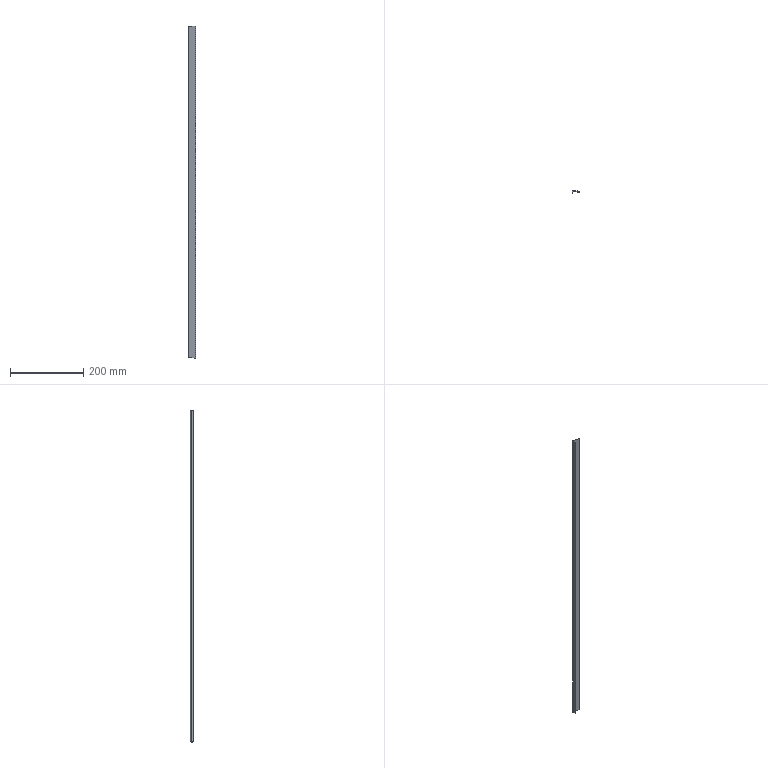Part | STEP file | 750078466 | 1 solid | 10 faces | box 19.319 x 9.272 x 903.6 mm | volume 29323 mm3 | plane 8 | cylinder 2 | commonest cylinder face diameters 2.4 x1 4.8 x1
STEP:
#1=CARTESIAN_POINT('',(19.008,3.665,451.8));
#2=VERTEX_POINT('',#1);
#3=CARTESIAN_POINT('',(19.008,3.665,-451.8));
#4=VERTEX_POINT('',#3);
#5=CARTESIAN_POINT('',(19.008,3.665,451.8));
#6=DIRECTION('',(0.,0.,-1.));
#7=VECTOR('',#6,1000.);
#8=LINE('',#5,#7);
#9=EDGE_CURVE('',#2,#4,#8,.T.);
#10=ORIENTED_EDGE('',*,*,#9,.F.);
#11=CARTESIAN_POINT('',(2.711,8.031,451.8));
#12=VERTEX_POINT('',#11);
#13=CARTESIAN_POINT('',(-0.3106,8.841,451.8));
#14=DIRECTION('',(0.9659,-0.2588,0.));
#15=VECTOR('',#14,1000.);
#16=LINE('',#13,#15);
#17=EDGE_CURVE('',#12,#2,#16,.T.);
#18=ORIENTED_EDGE('',*,*,#17,.F.);
#19=CARTESIAN_POINT('',(2.711,8.031,-451.8));
#20=VERTEX_POINT('',#19);
#21=CARTESIAN_POINT('',(2.711,8.031,451.8));
#22=DIRECTION('',(0.,0.,1.));
#23=VECTOR('',#22,1000.);
#24=LINE('',#21,#23);
#25=EDGE_CURVE('',#20,#12,#24,.T.);
#26=ORIENTED_EDGE('',*,*,#25,.F.);
#27=CARTESIAN_POINT('',(-0.3106,8.841,-451.8));
#28=DIRECTION('',(-0.9659,0.2588,0.));
#29=VECTOR('',#28,1000.);
#30=LINE('',#27,#29);
#31=EDGE_CURVE('',#4,#20,#30,.T.);
#32=ORIENTED_EDGE('',*,*,#31,.F.);
#33=EDGE_LOOP('',(#10,#18,#26,#32));
#34=FACE_OUTER_BOUND('',#33,.T.);
#35=CARTESIAN_POINT('',(-0.3106,8.841,451.8));
#36=DIRECTION('',(0.2588,0.9659,0.));
#37=DIRECTION('',(-0.9659,0.2588,0.));
#38=AXIS2_PLACEMENT_3D('',#35,#36,#37);
#39=PLANE('',#38);
#40=ADVANCED_FACE('',(#34),#39,.F.);
#41=CARTESIAN_POINT('',(3.021,9.19,-451.8));
#42=VERTEX_POINT('',#41);
#43=CARTESIAN_POINT('',(0.,6.872,-451.8));
#44=VERTEX_POINT('',#43);
#45=CARTESIAN_POINT('',(2.4,6.872,-451.8));
#46=DIRECTION('',(0.,0.,1.));
#47=DIRECTION('',(-1.,0.,0.));
#48=AXIS2_PLACEMENT_3D('',#45,#46,#47);
#49=CIRCLE('',#48,2.4);
#50=EDGE_CURVE('',#42,#44,#49,.T.);
#51=ORIENTED_EDGE('',*,*,#50,.F.);
#52=CARTESIAN_POINT('',(19.319,4.824,-451.8));
#53=VERTEX_POINT('',#52);
#54=CARTESIAN_POINT('',(19.319,4.824,-451.8));
#55=DIRECTION('',(-0.9659,0.2588,0.));
#56=VECTOR('',#55,1000.);
#57=LINE('',#54,#56);
#58=EDGE_CURVE('',#53,#42,#57,.T.);
#59=ORIENTED_EDGE('',*,*,#58,.F.);
#60=CARTESIAN_POINT('',(19.008,3.665,-451.8));
#61=DIRECTION('',(0.2588,0.9659,0.));
#62=VECTOR('',#61,1000.);
#63=LINE('',#60,#62);
#64=EDGE_CURVE('',#4,#53,#63,.T.);
#65=ORIENTED_EDGE('',*,*,#64,.F.);
#66=ORIENTED_EDGE('',*,*,#31,.T.);
#67=CARTESIAN_POINT('',(1.2,6.872,-451.8));
#68=VERTEX_POINT('',#67);
#69=CARTESIAN_POINT('',(2.4,6.872,-451.8));
#70=DIRECTION('',(0.,0.,-1.));
#71=DIRECTION('',(-1.,0.,0.));
#72=AXIS2_PLACEMENT_3D('',#69,#70,#71);
#73=CIRCLE('',#72,1.2);
#74=EDGE_CURVE('',#68,#20,#73,.T.);
#75=ORIENTED_EDGE('',*,*,#74,.F.);
#76=CARTESIAN_POINT('',(1.2,0.,-451.8));
#77=VERTEX_POINT('',#76);
#78=CARTESIAN_POINT('',(1.2,0.,-451.8));
#79=DIRECTION('',(0.,1.,0.));
#80=VECTOR('',#79,1000.);
#81=LINE('',#78,#80);
#82=EDGE_CURVE('',#77,#68,#81,.T.);
#83=ORIENTED_EDGE('',*,*,#82,.F.);
#84=CARTESIAN_POINT('',(0.,0.,-451.8));
#85=VERTEX_POINT('',#84);
#86=CARTESIAN_POINT('',(0.,0.,-451.8));
#87=DIRECTION('',(-1.,0.,0.));
#88=VECTOR('',#87,1000.);
#89=LINE('',#86,#88);
#90=EDGE_CURVE('',#77,#85,#89,.T.);
#91=ORIENTED_EDGE('',*,*,#90,.T.);
#92=CARTESIAN_POINT('',(0.,0.,-451.8));
#93=DIRECTION('',(0.,-1.,0.));
#94=VECTOR('',#93,1000.);
#95=LINE('',#92,#94);
#96=EDGE_CURVE('',#44,#85,#95,.T.);
#97=ORIENTED_EDGE('',*,*,#96,.F.);
#98=EDGE_LOOP('',(#51,#59,#65,#66,#75,#83,#91,#97));
#99=FACE_OUTER_BOUND('',#98,.T.);
#100=CARTESIAN_POINT('',(0.,0.,-451.8));
#101=DIRECTION('',(0.,0.,1.));
#102=DIRECTION('',(1.,0.,0.));
#103=AXIS2_PLACEMENT_3D('',#100,#101,#102);
#104=PLANE('',#103);
#105=ADVANCED_FACE('',(#99),#104,.F.);
#106=ORIENTED_EDGE('',*,*,#64,.T.);
#107=CARTESIAN_POINT('',(19.319,4.824,451.8));
#108=VERTEX_POINT('',#107);
#109=CARTESIAN_POINT('',(19.319,4.824,451.8));
#110=DIRECTION('',(0.,0.,1.));
#111=VECTOR('',#110,1000.);
#112=LINE('',#109,#111);
#113=EDGE_CURVE('',#53,#108,#112,.T.);
#114=ORIENTED_EDGE('',*,*,#113,.T.);
#115=CARTESIAN_POINT('',(19.319,4.824,451.8));
#116=DIRECTION('',(-0.2588,-0.9659,0.));
#117=VECTOR('',#116,1000.);
#118=LINE('',#115,#117);
#119=EDGE_CURVE('',#108,#2,#118,.T.);
#120=ORIENTED_EDGE('',*,*,#119,.T.);
#121=ORIENTED_EDGE('',*,*,#9,.T.);
#122=EDGE_LOOP('',(#106,#114,#120,#121));
#123=FACE_OUTER_BOUND('',#122,.T.);
#124=CARTESIAN_POINT('',(19.319,4.824,451.8));
#125=DIRECTION('',(0.9659,-0.2588,0.));
#126=DIRECTION('',(0.2588,0.9659,0.));
#127=AXIS2_PLACEMENT_3D('',#124,#125,#126);
#128=PLANE('',#127);
#129=ADVANCED_FACE('',(#123),#128,.T.);
#130=ORIENTED_EDGE('',*,*,#17,.T.);
#131=ORIENTED_EDGE('',*,*,#119,.F.);
#132=CARTESIAN_POINT('',(3.021,9.19,451.8));
#133=VERTEX_POINT('',#132);
#134=CARTESIAN_POINT('',(19.319,4.824,451.8));
#135=DIRECTION('',(-0.9659,0.2588,0.));
#136=VECTOR('',#135,1000.);
#137=LINE('',#134,#136);
#138=EDGE_CURVE('',#108,#133,#137,.T.);
#139=ORIENTED_EDGE('',*,*,#138,.T.);
#140=CARTESIAN_POINT('',(0.,6.872,451.8));
#141=VERTEX_POINT('',#140);
#142=CARTESIAN_POINT('',(2.4,6.872,451.8));
#143=DIRECTION('',(0.,0.,1.));
#144=DIRECTION('',(-1.,0.,0.));
#145=AXIS2_PLACEMENT_3D('',#142,#143,#144);
#146=CIRCLE('',#145,2.4);
#147=EDGE_CURVE('',#133,#141,#146,.T.);
#148=ORIENTED_EDGE('',*,*,#147,.T.);
#149=CARTESIAN_POINT('',(0.,0.,451.8));
#150=VERTEX_POINT('',#149);
#151=CARTESIAN_POINT('',(0.,10.,451.8));
#152=DIRECTION('',(0.,-1.,0.));
#153=VECTOR('',#152,1000.);
#154=LINE('',#151,#153);
#155=EDGE_CURVE('',#141,#150,#154,.T.);
#156=ORIENTED_EDGE('',*,*,#155,.T.);
#157=CARTESIAN_POINT('',(1.2,0.,451.8));
#158=VERTEX_POINT('',#157);
#159=CARTESIAN_POINT('',(0.,0.,451.8));
#160=DIRECTION('',(1.,0.,0.));
#161=VECTOR('',#160,1000.);
#162=LINE('',#159,#161);
#163=EDGE_CURVE('',#150,#158,#162,.T.);
#164=ORIENTED_EDGE('',*,*,#163,.T.);
#165=CARTESIAN_POINT('',(1.2,6.872,451.8));
#166=VERTEX_POINT('',#165);
#167=CARTESIAN_POINT('',(1.2,10.,451.8));
#168=DIRECTION('',(0.,1.,0.));
#169=VECTOR('',#168,1000.);
#170=LINE('',#167,#169);
#171=EDGE_CURVE('',#158,#166,#170,.T.);
#172=ORIENTED_EDGE('',*,*,#171,.T.);
#173=CARTESIAN_POINT('',(2.4,6.872,451.8));
#174=DIRECTION('',(0.,0.,-1.));
#175=DIRECTION('',(-1.,0.,0.));
#176=AXIS2_PLACEMENT_3D('',#173,#174,#175);
#177=CIRCLE('',#176,1.2);
#178=EDGE_CURVE('',#166,#12,#177,.T.);
#179=ORIENTED_EDGE('',*,*,#178,.T.);
#180=EDGE_LOOP('',(#130,#131,#139,#148,#156,#164,#172,#179));
#181=FACE_OUTER_BOUND('',#180,.T.);
#182=CARTESIAN_POINT('',(0.,10.,451.8));
#183=DIRECTION('',(0.,0.,1.));
#184=DIRECTION('',(1.,0.,0.));
#185=AXIS2_PLACEMENT_3D('',#182,#183,#184);
#186=PLANE('',#185);
#187=ADVANCED_FACE('',(#181),#186,.T.);
#188=ORIENTED_EDGE('',*,*,#25,.T.);
#189=ORIENTED_EDGE('',*,*,#178,.F.);
#190=CARTESIAN_POINT('',(1.2,6.872,451.8));
#191=DIRECTION('',(0.,0.,1.));
#192=VECTOR('',#191,1000.);
#193=LINE('',#190,#192);
#194=EDGE_CURVE('',#68,#166,#193,.T.);
#195=ORIENTED_EDGE('',*,*,#194,.F.);
#196=ORIENTED_EDGE('',*,*,#74,.T.);
#197=EDGE_LOOP('',(#188,#189,#195,#196));
#198=FACE_OUTER_BOUND('',#197,.T.);
#199=CARTESIAN_POINT('',(2.4,6.872,451.8));
#200=DIRECTION('',(0.,0.,-1.));
#201=DIRECTION('',(-1.,0.,0.));
#202=AXIS2_PLACEMENT_3D('',#199,#200,#201);
#203=CYLINDRICAL_SURFACE('',#202,1.2);
#204=ADVANCED_FACE('',(#198),#203,.F.);
#205=ORIENTED_EDGE('',*,*,#155,.F.);
#206=CARTESIAN_POINT('',(0.,6.872,451.8));
#207=DIRECTION('',(0.,0.,-1.));
#208=VECTOR('',#207,1000.);
#209=LINE('',#206,#208);
#210=EDGE_CURVE('',#141,#44,#209,.T.);
#211=ORIENTED_EDGE('',*,*,#210,.T.);
#212=ORIENTED_EDGE('',*,*,#96,.T.);
#213=CARTESIAN_POINT('',(0.,0.,451.8));
#214=DIRECTION('',(0.,0.,1.));
#215=VECTOR('',#214,1000.);
#216=LINE('',#213,#215);
#217=EDGE_CURVE('',#85,#150,#216,.T.);
#218=ORIENTED_EDGE('',*,*,#217,.T.);
#219=EDGE_LOOP('',(#205,#211,#212,#218));
#220=FACE_OUTER_BOUND('',#219,.T.);
#221=CARTESIAN_POINT('',(0.,0.,451.8));
#222=DIRECTION('',(-1.,0.,0.));
#223=DIRECTION('',(0.,0.,1.));
#224=AXIS2_PLACEMENT_3D('',#221,#222,#223);
#225=PLANE('',#224);
#226=ADVANCED_FACE('',(#220),#225,.T.);
#227=ORIENTED_EDGE('',*,*,#147,.F.);
#228=CARTESIAN_POINT('',(3.021,9.19,451.8));
#229=DIRECTION('',(0.,0.,-1.));
#230=VECTOR('',#229,1000.);
#231=LINE('',#228,#230);
#232=EDGE_CURVE('',#133,#42,#231,.T.);
#233=ORIENTED_EDGE('',*,*,#232,.T.);
#234=ORIENTED_EDGE('',*,*,#50,.T.);
#235=ORIENTED_EDGE('',*,*,#210,.F.);
#236=EDGE_LOOP('',(#227,#233,#234,#235));
#237=FACE_OUTER_BOUND('',#236,.T.);
#238=CARTESIAN_POINT('',(2.4,6.872,451.8));
#239=DIRECTION('',(0.,0.,-1.));
#240=DIRECTION('',(-1.,0.,0.));
#241=AXIS2_PLACEMENT_3D('',#238,#239,#240);
#242=CYLINDRICAL_SURFACE('',#241,2.4);
#243=ADVANCED_FACE('',(#237),#242,.T.);
#244=ORIENTED_EDGE('',*,*,#138,.F.);
#245=ORIENTED_EDGE('',*,*,#113,.F.);
#246=ORIENTED_EDGE('',*,*,#58,.T.);
#247=ORIENTED_EDGE('',*,*,#232,.F.);
#248=EDGE_LOOP('',(#244,#245,#246,#247));
#249=FACE_OUTER_BOUND('',#248,.T.);
#250=CARTESIAN_POINT('',(0.,10.,451.8));
#251=DIRECTION('',(0.2588,0.9659,0.));
#252=DIRECTION('',(-0.9659,0.2588,0.));
#253=AXIS2_PLACEMENT_3D('',#250,#251,#252);
#254=PLANE('',#253);
#255=ADVANCED_FACE('',(#249),#254,.T.);
#256=ORIENTED_EDGE('',*,*,#194,.T.);
#257=ORIENTED_EDGE('',*,*,#171,.F.);
#258=CARTESIAN_POINT('',(1.2,0.,451.8));
#259=DIRECTION('',(0.,0.,1.));
#260=VECTOR('',#259,1000.);
#261=LINE('',#258,#260);
#262=EDGE_CURVE('',#77,#158,#261,.T.);
#263=ORIENTED_EDGE('',*,*,#262,.F.);
#264=ORIENTED_EDGE('',*,*,#82,.T.);
#265=EDGE_LOOP('',(#256,#257,#263,#264));
#266=FACE_OUTER_BOUND('',#265,.T.);
#267=CARTESIAN_POINT('',(1.2,0.,451.8));
#268=DIRECTION('',(-1.,0.,0.));
#269=DIRECTION('',(0.,0.,1.));
#270=AXIS2_PLACEMENT_3D('',#267,#268,#269);
#271=PLANE('',#270);
#272=ADVANCED_FACE('',(#266),#271,.F.);
#273=ORIENTED_EDGE('',*,*,#163,.F.);
#274=ORIENTED_EDGE('',*,*,#217,.F.);
#275=ORIENTED_EDGE('',*,*,#90,.F.);
#276=ORIENTED_EDGE('',*,*,#262,.T.);
#277=EDGE_LOOP('',(#273,#274,#275,#276));
#278=FACE_OUTER_BOUND('',#277,.T.);
#279=CARTESIAN_POINT('',(0.,0.,451.8));
#280=DIRECTION('',(0.,1.,0.));
#281=DIRECTION('',(0.,0.,1.));
#282=AXIS2_PLACEMENT_3D('',#279,#280,#281);
#283=PLANE('',#282);
#284=ADVANCED_FACE('',(#278),#283,.F.);
#285=CLOSED_SHELL('',(#40,#105,#129,#187,#204,#226,#243,#255,#272,#284));
#286=MANIFOLD_SOLID_BREP('',#285);
#287=CARTESIAN_POINT('',(0.,0.,0.));
#288=DIRECTION('',(0.,0.,1.));
#289=DIRECTION('',(1.,0.,0.));
#290=AXIS2_PLACEMENT_3D('',#287,#288,#289);
#291=(LENGTH_UNIT()NAMED_UNIT(*)SI_UNIT(.MILLI.,.METRE.));
#292=UNCERTAINTY_MEASURE_WITH_UNIT(LENGTH_MEASURE(0.00001),#291,'','');
#293=(NAMED_UNIT(*)PLANE_ANGLE_UNIT()SI_UNIT($,.RADIAN.));
#294=(NAMED_UNIT(*)SI_UNIT($,.STERADIAN.)SOLID_ANGLE_UNIT());
#295=(GEOMETRIC_REPRESENTATION_CONTEXT(3)GLOBAL_UNCERTAINTY_ASSIGNED_CONTEXT((#292))GLOBAL_UNIT_ASSIGNED_CONTEXT((#291,#293,#294))REPRESENTATION_CONTEXT('',''));
#296=ADVANCED_BREP_SHAPE_REPRESENTATION('',(#286,#290),#295);